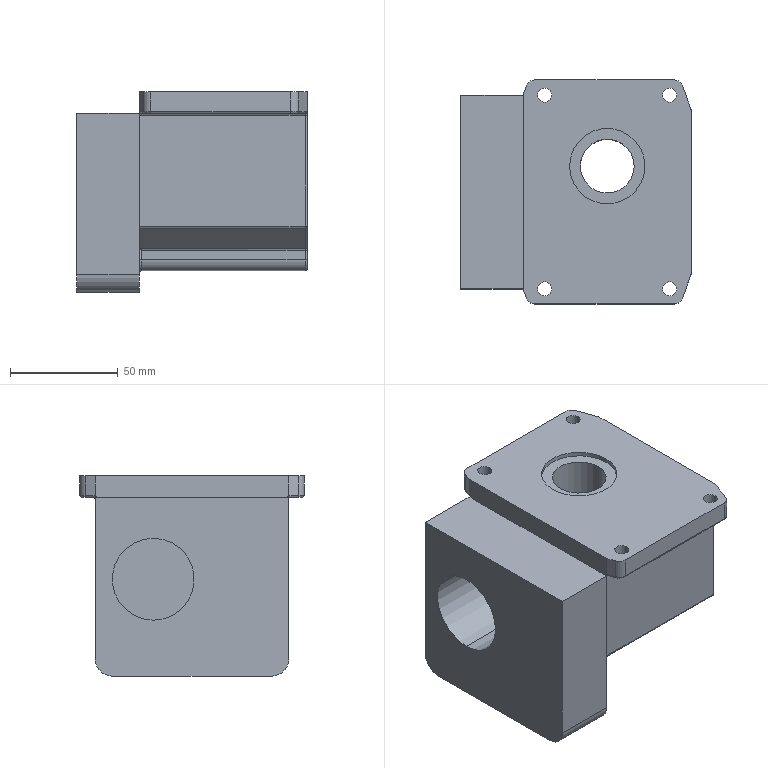Part | STEP file | 0228_Z_Gearhead_5GN120RH1 | 1 solid | 105 faces | box 107 x 104 x 93 mm | volume 637231 mm3 | cylinder 53 | plane 28 | torus 12 | sphere 7 | spline 5 | commonest cylinder face diameters 2 x32 6.5 x8 8 x4 16.4 x2 25 x2 35 x2